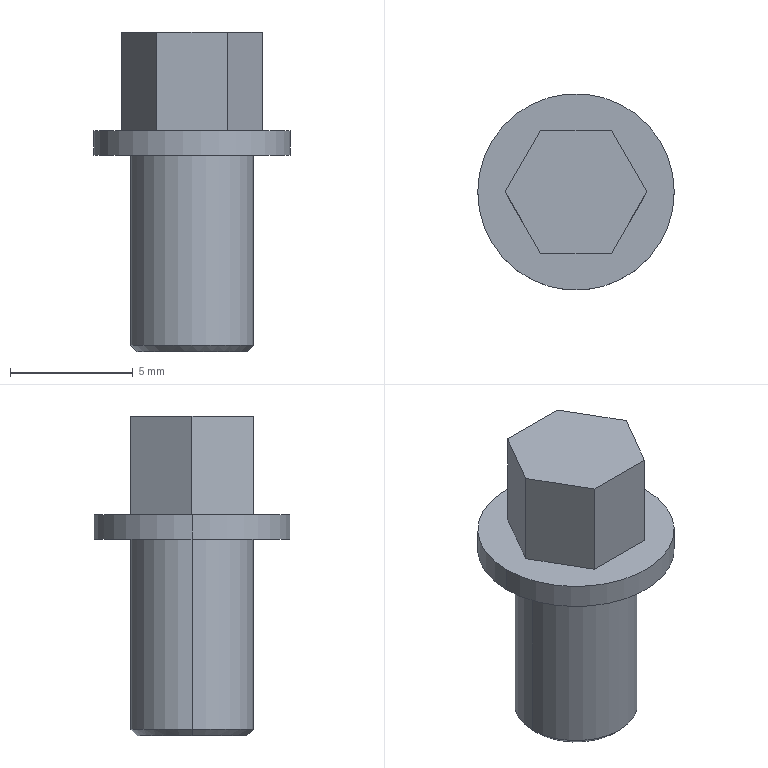Part | SolidWorks | features BaseBody 1 | 1 solid | 16 faces | box 8 x 8 x 13 mm | volume 293.473 mm3 | plane 10 | cylinder 4 | cone 2 | commonest cylinder face diameters 5 x2 8 x2
STEP:
#1=CARTESIAN_POINT('',(2.25,0.,-8.));
#2=VERTEX_POINT('',#1);
#3=CARTESIAN_POINT('',(-2.25,0.,-8.));
#4=VERTEX_POINT('',#3);
#5=CARTESIAN_POINT('',(0.,0.,-8.));
#6=DIRECTION('',(0.,0.,1.));
#7=DIRECTION('',(1.,0.,0.));
#8=AXIS2_PLACEMENT_3D('',#5,#6,#7);
#9=CIRCLE('',#8,2.25);
#10=EDGE_CURVE('',#2,#4,#9,.T.);
#11=ORIENTED_EDGE('',*,*,#10,.T.);
#12=CARTESIAN_POINT('',(-2.5,0.,-7.75));
#13=VERTEX_POINT('',#12);
#14=CARTESIAN_POINT('',(-2.375,0.,-7.875));
#15=DIRECTION('',(-0.7071,0.,0.7071));
#16=VECTOR('',#15,1000.);
#17=LINE('',#14,#16);
#18=EDGE_CURVE('',#4,#13,#17,.T.);
#19=ORIENTED_EDGE('',*,*,#18,.T.);
#20=CARTESIAN_POINT('',(2.5,0.,-7.75));
#21=VERTEX_POINT('',#20);
#22=CARTESIAN_POINT('',(0.,0.,-7.75));
#23=DIRECTION('',(0.,0.,-1.));
#24=DIRECTION('',(1.,0.,0.));
#25=AXIS2_PLACEMENT_3D('',#22,#23,#24);
#26=CIRCLE('',#25,2.5);
#27=EDGE_CURVE('',#13,#21,#26,.T.);
#28=ORIENTED_EDGE('',*,*,#27,.T.);
#29=CARTESIAN_POINT('',(2.375,0.,-7.875));
#30=DIRECTION('',(0.7071,0.,0.7071));
#31=VECTOR('',#30,1000.);
#32=LINE('',#29,#31);
#33=EDGE_CURVE('',#2,#21,#32,.T.);
#34=ORIENTED_EDGE('',*,*,#33,.F.);
#35=EDGE_LOOP('',(#11,#19,#28,#34));
#36=FACE_OUTER_BOUND('',#35,.T.);
#37=CARTESIAN_POINT('',(0.,0.,-7.875));
#38=DIRECTION('',(0.,0.,1.));
#39=DIRECTION('',(1.,0.,0.));
#40=AXIS2_PLACEMENT_3D('',#37,#38,#39);
#41=CONICAL_SURFACE('',#40,2.375,0.7854);
#42=ADVANCED_FACE('',(#36),#41,.T.);
#43=ORIENTED_EDGE('',*,*,#27,.F.);
#44=CARTESIAN_POINT('',(-2.5,0.,0.));
#45=VERTEX_POINT('',#44);
#46=CARTESIAN_POINT('',(-2.5,0.,0.));
#47=DIRECTION('',(0.,0.,1.));
#48=VECTOR('',#47,1000.);
#49=LINE('',#46,#48);
#50=EDGE_CURVE('',#13,#45,#49,.T.);
#51=ORIENTED_EDGE('',*,*,#50,.T.);
#52=CARTESIAN_POINT('',(2.5,0.,0.));
#53=VERTEX_POINT('',#52);
#54=CARTESIAN_POINT('',(0.,0.,0.));
#55=DIRECTION('',(0.,0.,1.));
#56=DIRECTION('',(1.,0.,0.));
#57=AXIS2_PLACEMENT_3D('',#54,#55,#56);
#58=CIRCLE('',#57,2.5);
#59=EDGE_CURVE('',#53,#45,#58,.T.);
#60=ORIENTED_EDGE('',*,*,#59,.F.);
#61=CARTESIAN_POINT('',(2.5,0.,0.));
#62=DIRECTION('',(0.,0.,1.));
#63=VECTOR('',#62,1000.);
#64=LINE('',#61,#63);
#65=EDGE_CURVE('',#21,#53,#64,.T.);
#66=ORIENTED_EDGE('',*,*,#65,.F.);
#67=EDGE_LOOP('',(#43,#51,#60,#66));
#68=FACE_OUTER_BOUND('',#67,.T.);
#69=CARTESIAN_POINT('',(0.,0.,0.));
#70=DIRECTION('',(0.,0.,1.));
#71=DIRECTION('',(1.,0.,0.));
#72=AXIS2_PLACEMENT_3D('',#69,#70,#71);
#73=CYLINDRICAL_SURFACE('',#72,2.5);
#74=ADVANCED_FACE('',(#68),#73,.T.);
#75=CARTESIAN_POINT('',(4.,0.,1.));
#76=VERTEX_POINT('',#75);
#77=CARTESIAN_POINT('',(-4.,0.,1.));
#78=VERTEX_POINT('',#77);
#79=CARTESIAN_POINT('',(0.,0.,1.));
#80=DIRECTION('',(0.,0.,1.));
#81=DIRECTION('',(-1.,0.,0.));
#82=AXIS2_PLACEMENT_3D('',#79,#80,#81);
#83=CIRCLE('',#82,4.);
#84=EDGE_CURVE('',#76,#78,#83,.T.);
#85=ORIENTED_EDGE('',*,*,#84,.F.);
#86=CARTESIAN_POINT('',(4.,0.,0.));
#87=VERTEX_POINT('',#86);
#88=CARTESIAN_POINT('',(4.,0.,0.));
#89=DIRECTION('',(0.,0.,-1.));
#90=VECTOR('',#89,1000.);
#91=LINE('',#88,#90);
#92=EDGE_CURVE('',#76,#87,#91,.T.);
#93=ORIENTED_EDGE('',*,*,#92,.T.);
#94=CARTESIAN_POINT('',(-4.,0.,0.));
#95=VERTEX_POINT('',#94);
#96=CARTESIAN_POINT('',(0.,0.,0.));
#97=DIRECTION('',(0.,0.,-1.));
#98=DIRECTION('',(-1.,0.,0.));
#99=AXIS2_PLACEMENT_3D('',#96,#97,#98);
#100=CIRCLE('',#99,4.);
#101=EDGE_CURVE('',#95,#87,#100,.T.);
#102=ORIENTED_EDGE('',*,*,#101,.F.);
#103=CARTESIAN_POINT('',(-4.,0.,0.));
#104=DIRECTION('',(0.,0.,-1.));
#105=VECTOR('',#104,1000.);
#106=LINE('',#103,#105);
#107=EDGE_CURVE('',#78,#95,#106,.T.);
#108=ORIENTED_EDGE('',*,*,#107,.F.);
#109=EDGE_LOOP('',(#85,#93,#102,#108));
#110=FACE_OUTER_BOUND('',#109,.T.);
#111=CARTESIAN_POINT('',(0.,0.,0.));
#112=DIRECTION('',(0.,0.,-1.));
#113=DIRECTION('',(-1.,0.,0.));
#114=AXIS2_PLACEMENT_3D('',#111,#112,#113);
#115=CYLINDRICAL_SURFACE('',#114,4.);
#116=ADVANCED_FACE('',(#110),#115,.T.);
#117=ORIENTED_EDGE('',*,*,#10,.F.);
#118=CARTESIAN_POINT('',(0.,0.,-8.));
#119=DIRECTION('',(0.,0.,1.));
#120=DIRECTION('',(1.,0.,0.));
#121=AXIS2_PLACEMENT_3D('',#118,#119,#120);
#122=CIRCLE('',#121,2.25);
#123=EDGE_CURVE('',#4,#2,#122,.T.);
#124=ORIENTED_EDGE('',*,*,#123,.F.);
#125=EDGE_LOOP('',(#117,#124));
#126=FACE_OUTER_BOUND('',#125,.T.);
#127=CARTESIAN_POINT('',(0.,0.,-8.));
#128=DIRECTION('',(0.,0.,1.));
#129=DIRECTION('',(1.,0.,0.));
#130=AXIS2_PLACEMENT_3D('',#127,#128,#129);
#131=PLANE('',#130);
#132=ADVANCED_FACE('',(#126),#131,.F.);
#133=CARTESIAN_POINT('',(-1.443,-2.5,1.));
#134=VERTEX_POINT('',#133);
#135=CARTESIAN_POINT('',(-2.887,0.,1.));
#136=VERTEX_POINT('',#135);
#137=CARTESIAN_POINT('',(-2.526,-0.625,1.));
#138=DIRECTION('',(-0.5,0.866,0.));
#139=VECTOR('',#138,1000.);
#140=LINE('',#137,#139);
#141=EDGE_CURVE('',#134,#136,#140,.T.);
#142=ORIENTED_EDGE('',*,*,#141,.F.);
#143=CARTESIAN_POINT('',(-1.443,-2.5,5.));
#144=VERTEX_POINT('',#143);
#145=CARTESIAN_POINT('',(-1.443,-2.5,1.));
#146=DIRECTION('',(0.,0.,1.));
#147=VECTOR('',#146,1000.);
#148=LINE('',#145,#147);
#149=EDGE_CURVE('',#134,#144,#148,.T.);
#150=ORIENTED_EDGE('',*,*,#149,.T.);
#151=CARTESIAN_POINT('',(-2.887,0.,5.));
#152=VERTEX_POINT('',#151);
#153=CARTESIAN_POINT('',(-1.443,-2.5,5.));
#154=DIRECTION('',(0.5,-0.866,0.));
#155=VECTOR('',#154,1000.);
#156=LINE('',#153,#155);
#157=EDGE_CURVE('',#152,#144,#156,.T.);
#158=ORIENTED_EDGE('',*,*,#157,.F.);
#159=CARTESIAN_POINT('',(-2.887,0.,1.));
#160=DIRECTION('',(0.,0.,1.));
#161=VECTOR('',#160,1000.);
#162=LINE('',#159,#161);
#163=EDGE_CURVE('',#136,#152,#162,.T.);
#164=ORIENTED_EDGE('',*,*,#163,.F.);
#165=EDGE_LOOP('',(#142,#150,#158,#164));
#166=FACE_OUTER_BOUND('',#165,.T.);
#167=CARTESIAN_POINT('',(-2.887,0.,1.));
#168=DIRECTION('',(-0.866,-0.5,0.));
#169=DIRECTION('',(-0.5,0.866,0.));
#170=AXIS2_PLACEMENT_3D('',#167,#168,#169);
#171=PLANE('',#170);
#172=ADVANCED_FACE('',(#166),#171,.T.);
#173=CARTESIAN_POINT('',(-1.443,2.5,1.));
#174=VERTEX_POINT('',#173);
#175=CARTESIAN_POINT('',(-1.804,1.875,1.));
#176=DIRECTION('',(0.5,0.866,0.));
#177=VECTOR('',#176,1000.);
#178=LINE('',#175,#177);
#179=EDGE_CURVE('',#136,#174,#178,.T.);
#180=ORIENTED_EDGE('',*,*,#179,.F.);
#181=ORIENTED_EDGE('',*,*,#163,.T.);
#182=CARTESIAN_POINT('',(-1.443,2.5,5.));
#183=VERTEX_POINT('',#182);
#184=CARTESIAN_POINT('',(-2.887,0.,5.));
#185=DIRECTION('',(-0.5,-0.866,0.));
#186=VECTOR('',#185,1000.);
#187=LINE('',#184,#186);
#188=EDGE_CURVE('',#183,#152,#187,.T.);
#189=ORIENTED_EDGE('',*,*,#188,.F.);
#190=CARTESIAN_POINT('',(-1.443,2.5,1.));
#191=DIRECTION('',(0.,0.,1.));
#192=VECTOR('',#191,1000.);
#193=LINE('',#190,#192);
#194=EDGE_CURVE('',#174,#183,#193,.T.);
#195=ORIENTED_EDGE('',*,*,#194,.F.);
#196=EDGE_LOOP('',(#180,#181,#189,#195));
#197=FACE_OUTER_BOUND('',#196,.T.);
#198=CARTESIAN_POINT('',(-1.443,2.5,1.));
#199=DIRECTION('',(-0.866,0.5,0.));
#200=DIRECTION('',(0.,0.,1.));
#201=AXIS2_PLACEMENT_3D('',#198,#199,#200);
#202=PLANE('',#201);
#203=ADVANCED_FACE('',(#197),#202,.T.);
#204=CARTESIAN_POINT('',(1.443,2.5,1.));
#205=VERTEX_POINT('',#204);
#206=CARTESIAN_POINT('',(0.7217,2.5,1.));
#207=DIRECTION('',(1.,0.,0.));
#208=VECTOR('',#207,1000.);
#209=LINE('',#206,#208);
#210=EDGE_CURVE('',#174,#205,#209,.T.);
#211=ORIENTED_EDGE('',*,*,#210,.F.);
#212=ORIENTED_EDGE('',*,*,#194,.T.);
#213=CARTESIAN_POINT('',(1.443,2.5,5.));
#214=VERTEX_POINT('',#213);
#215=CARTESIAN_POINT('',(-1.443,2.5,5.));
#216=DIRECTION('',(-1.,0.,0.));
#217=VECTOR('',#216,1000.);
#218=LINE('',#215,#217);
#219=EDGE_CURVE('',#214,#183,#218,.T.);
#220=ORIENTED_EDGE('',*,*,#219,.F.);
#221=CARTESIAN_POINT('',(1.443,2.5,1.));
#222=DIRECTION('',(0.,0.,1.));
#223=VECTOR('',#222,1000.);
#224=LINE('',#221,#223);
#225=EDGE_CURVE('',#205,#214,#224,.T.);
#226=ORIENTED_EDGE('',*,*,#225,.F.);
#227=EDGE_LOOP('',(#211,#212,#220,#226));
#228=FACE_OUTER_BOUND('',#227,.T.);
#229=CARTESIAN_POINT('',(1.443,2.5,1.));
#230=DIRECTION('',(0.,1.,0.));
#231=DIRECTION('',(1.,0.,0.));
#232=AXIS2_PLACEMENT_3D('',#229,#230,#231);
#233=PLANE('',#232);
#234=ADVANCED_FACE('',(#228),#233,.T.);
#235=CARTESIAN_POINT('',(2.887,0.,1.));
#236=VERTEX_POINT('',#235);
#237=CARTESIAN_POINT('',(2.526,0.625,1.));
#238=DIRECTION('',(0.5,-0.866,0.));
#239=VECTOR('',#238,1000.);
#240=LINE('',#237,#239);
#241=EDGE_CURVE('',#205,#236,#240,.T.);
#242=ORIENTED_EDGE('',*,*,#241,.F.);
#243=ORIENTED_EDGE('',*,*,#225,.T.);
#244=CARTESIAN_POINT('',(2.887,0.,5.));
#245=VERTEX_POINT('',#244);
#246=CARTESIAN_POINT('',(1.443,2.5,5.));
#247=DIRECTION('',(-0.5,0.866,0.));
#248=VECTOR('',#247,1000.);
#249=LINE('',#246,#248);
#250=EDGE_CURVE('',#245,#214,#249,.T.);
#251=ORIENTED_EDGE('',*,*,#250,.F.);
#252=CARTESIAN_POINT('',(2.887,0.,1.));
#253=DIRECTION('',(0.,0.,1.));
#254=VECTOR('',#253,1000.);
#255=LINE('',#252,#254);
#256=EDGE_CURVE('',#236,#245,#255,.T.);
#257=ORIENTED_EDGE('',*,*,#256,.F.);
#258=EDGE_LOOP('',(#242,#243,#251,#257));
#259=FACE_OUTER_BOUND('',#258,.T.);
#260=CARTESIAN_POINT('',(2.887,0.,1.));
#261=DIRECTION('',(0.866,0.5,0.));
#262=DIRECTION('',(0.,0.,-1.));
#263=AXIS2_PLACEMENT_3D('',#260,#261,#262);
#264=PLANE('',#263);
#265=ADVANCED_FACE('',(#259),#264,.T.);
#266=CARTESIAN_POINT('',(1.443,-2.5,1.));
#267=VERTEX_POINT('',#266);
#268=CARTESIAN_POINT('',(1.804,-1.875,1.));
#269=DIRECTION('',(-0.5,-0.866,0.));
#270=VECTOR('',#269,1000.);
#271=LINE('',#268,#270);
#272=EDGE_CURVE('',#236,#267,#271,.T.);
#273=ORIENTED_EDGE('',*,*,#272,.F.);
#274=ORIENTED_EDGE('',*,*,#256,.T.);
#275=CARTESIAN_POINT('',(1.443,-2.5,5.));
#276=VERTEX_POINT('',#275);
#277=CARTESIAN_POINT('',(2.887,0.,5.));
#278=DIRECTION('',(0.5,0.866,0.));
#279=VECTOR('',#278,1000.);
#280=LINE('',#277,#279);
#281=EDGE_CURVE('',#276,#245,#280,.T.);
#282=ORIENTED_EDGE('',*,*,#281,.F.);
#283=CARTESIAN_POINT('',(1.443,-2.5,1.));
#284=DIRECTION('',(0.,0.,1.));
#285=VECTOR('',#284,1000.);
#286=LINE('',#283,#285);
#287=EDGE_CURVE('',#267,#276,#286,.T.);
#288=ORIENTED_EDGE('',*,*,#287,.F.);
#289=EDGE_LOOP('',(#273,#274,#282,#288));
#290=FACE_OUTER_BOUND('',#289,.T.);
#291=CARTESIAN_POINT('',(1.443,-2.5,1.));
#292=DIRECTION('',(0.866,-0.5,0.));
#293=DIRECTION('',(0.,0.,-1.));
#294=AXIS2_PLACEMENT_3D('',#291,#292,#293);
#295=PLANE('',#294);
#296=ADVANCED_FACE('',(#290),#295,.T.);
#297=CARTESIAN_POINT('',(-0.7217,-2.5,1.));
#298=DIRECTION('',(-1.,0.,0.));
#299=VECTOR('',#298,1000.);
#300=LINE('',#297,#299);
#301=EDGE_CURVE('',#267,#134,#300,.T.);
#302=ORIENTED_EDGE('',*,*,#301,.F.);
#303=ORIENTED_EDGE('',*,*,#287,.T.);
#304=CARTESIAN_POINT('',(1.443,-2.5,5.));
#305=DIRECTION('',(1.,0.,0.));
#306=VECTOR('',#305,1000.);
#307=LINE('',#304,#306);
#308=EDGE_CURVE('',#144,#276,#307,.T.);
#309=ORIENTED_EDGE('',*,*,#308,.F.);
#310=ORIENTED_EDGE('',*,*,#149,.F.);
#311=EDGE_LOOP('',(#302,#303,#309,#310));
#312=FACE_OUTER_BOUND('',#311,.T.);
#313=CARTESIAN_POINT('',(-1.443,-2.5,1.));
#314=DIRECTION('',(0.,-1.,0.));
#315=DIRECTION('',(-1.,0.,0.));
#316=AXIS2_PLACEMENT_3D('',#313,#314,#315);
#317=PLANE('',#316);
#318=ADVANCED_FACE('',(#312),#317,.T.);
#319=ORIENTED_EDGE('',*,*,#308,.T.);
#320=ORIENTED_EDGE('',*,*,#281,.T.);
#321=ORIENTED_EDGE('',*,*,#250,.T.);
#322=ORIENTED_EDGE('',*,*,#219,.T.);
#323=ORIENTED_EDGE('',*,*,#188,.T.);
#324=ORIENTED_EDGE('',*,*,#157,.T.);
#325=EDGE_LOOP('',(#319,#320,#321,#322,#323,#324));
#326=FACE_OUTER_BOUND('',#325,.T.);
#327=CARTESIAN_POINT('',(0.,0.,5.));
#328=DIRECTION('',(0.,0.,1.));
#329=DIRECTION('',(1.,0.,0.));
#330=AXIS2_PLACEMENT_3D('',#327,#328,#329);
#331=PLANE('',#330);
#332=ADVANCED_FACE('',(#326),#331,.T.);
#333=ORIENTED_EDGE('',*,*,#59,.T.);
#334=CARTESIAN_POINT('',(0.,0.,0.));
#335=DIRECTION('',(0.,0.,1.));
#336=DIRECTION('',(1.,0.,0.));
#337=AXIS2_PLACEMENT_3D('',#334,#335,#336);
#338=CIRCLE('',#337,2.5);
#339=EDGE_CURVE('',#45,#53,#338,.T.);
#340=ORIENTED_EDGE('',*,*,#339,.T.);
#341=EDGE_LOOP('',(#333,#340));
#342=FACE_BOUND('',#341,.T.);
#343=ORIENTED_EDGE('',*,*,#101,.T.);
#344=CARTESIAN_POINT('',(0.,0.,0.));
#345=DIRECTION('',(0.,0.,-1.));
#346=DIRECTION('',(-1.,0.,0.));
#347=AXIS2_PLACEMENT_3D('',#344,#345,#346);
#348=CIRCLE('',#347,4.);
#349=EDGE_CURVE('',#87,#95,#348,.T.);
#350=ORIENTED_EDGE('',*,*,#349,.T.);
#351=EDGE_LOOP('',(#343,#350));
#352=FACE_OUTER_BOUND('',#351,.T.);
#353=CARTESIAN_POINT('',(0.,0.,0.));
#354=DIRECTION('',(0.,0.,1.));
#355=DIRECTION('',(1.,0.,0.));
#356=AXIS2_PLACEMENT_3D('',#353,#354,#355);
#357=PLANE('',#356);
#358=ADVANCED_FACE('',(#342,#352),#357,.F.);
#359=ORIENTED_EDGE('',*,*,#141,.T.);
#360=ORIENTED_EDGE('',*,*,#179,.T.);
#361=ORIENTED_EDGE('',*,*,#210,.T.);
#362=ORIENTED_EDGE('',*,*,#241,.T.);
#363=ORIENTED_EDGE('',*,*,#272,.T.);
#364=ORIENTED_EDGE('',*,*,#301,.T.);
#365=EDGE_LOOP('',(#359,#360,#361,#362,#363,#364));
#366=FACE_BOUND('',#365,.T.);
#367=CARTESIAN_POINT('',(0.,0.,1.));
#368=DIRECTION('',(0.,0.,1.));
#369=DIRECTION('',(-1.,0.,0.));
#370=AXIS2_PLACEMENT_3D('',#367,#368,#369);
#371=CIRCLE('',#370,4.);
#372=EDGE_CURVE('',#78,#76,#371,.T.);
#373=ORIENTED_EDGE('',*,*,#372,.T.);
#374=ORIENTED_EDGE('',*,*,#84,.T.);
#375=EDGE_LOOP('',(#373,#374));
#376=FACE_OUTER_BOUND('',#375,.T.);
#377=CARTESIAN_POINT('',(0.,0.,1.));
#378=DIRECTION('',(0.,0.,1.));
#379=DIRECTION('',(1.,0.,0.));
#380=AXIS2_PLACEMENT_3D('',#377,#378,#379);
#381=PLANE('',#380);
#382=ADVANCED_FACE('',(#366,#376),#381,.T.);
#383=ORIENTED_EDGE('',*,*,#92,.F.);
#384=ORIENTED_EDGE('',*,*,#372,.F.);
#385=ORIENTED_EDGE('',*,*,#107,.T.);
#386=ORIENTED_EDGE('',*,*,#349,.F.);
#387=EDGE_LOOP('',(#383,#384,#385,#386));
#388=FACE_OUTER_BOUND('',#387,.T.);
#389=CARTESIAN_POINT('',(0.,0.,0.));
#390=DIRECTION('',(0.,0.,-1.));
#391=DIRECTION('',(-1.,0.,0.));
#392=AXIS2_PLACEMENT_3D('',#389,#390,#391);
#393=CYLINDRICAL_SURFACE('',#392,4.);
#394=ADVANCED_FACE('',(#388),#393,.T.);
#395=ORIENTED_EDGE('',*,*,#50,.F.);
#396=CARTESIAN_POINT('',(0.,0.,-7.75));
#397=DIRECTION('',(0.,0.,-1.));
#398=DIRECTION('',(1.,0.,0.));
#399=AXIS2_PLACEMENT_3D('',#396,#397,#398);
#400=CIRCLE('',#399,2.5);
#401=EDGE_CURVE('',#21,#13,#400,.T.);
#402=ORIENTED_EDGE('',*,*,#401,.F.);
#403=ORIENTED_EDGE('',*,*,#65,.T.);
#404=ORIENTED_EDGE('',*,*,#339,.F.);
#405=EDGE_LOOP('',(#395,#402,#403,#404));
#406=FACE_OUTER_BOUND('',#405,.T.);
#407=CARTESIAN_POINT('',(0.,0.,0.));
#408=DIRECTION('',(0.,0.,1.));
#409=DIRECTION('',(1.,0.,0.));
#410=AXIS2_PLACEMENT_3D('',#407,#408,#409);
#411=CYLINDRICAL_SURFACE('',#410,2.5);
#412=ADVANCED_FACE('',(#406),#411,.T.);
#413=ORIENTED_EDGE('',*,*,#18,.F.);
#414=ORIENTED_EDGE('',*,*,#123,.T.);
#415=ORIENTED_EDGE('',*,*,#33,.T.);
#416=ORIENTED_EDGE('',*,*,#401,.T.);
#417=EDGE_LOOP('',(#413,#414,#415,#416));
#418=FACE_OUTER_BOUND('',#417,.T.);
#419=CARTESIAN_POINT('',(0.,0.,-7.875));
#420=DIRECTION('',(0.,0.,1.));
#421=DIRECTION('',(1.,0.,0.));
#422=AXIS2_PLACEMENT_3D('',#419,#420,#421);
#423=CONICAL_SURFACE('',#422,2.375,0.7854);
#424=ADVANCED_FACE('',(#418),#423,.T.);
#425=CLOSED_SHELL('',(#42,#74,#116,#132,#172,#203,#234,#265,#296,#318,#332,#358,#382,#394,#412,#424));
#426=MANIFOLD_SOLID_BREP('',#425);
#427=CARTESIAN_POINT('',(0.,0.,0.));
#428=DIRECTION('',(0.,0.,1.));
#429=DIRECTION('',(1.,0.,0.));
#430=AXIS2_PLACEMENT_3D('',#427,#428,#429);
#431=(LENGTH_UNIT()NAMED_UNIT(*)SI_UNIT(.MILLI.,.METRE.));
#432=UNCERTAINTY_MEASURE_WITH_UNIT(LENGTH_MEASURE(0.00001),#431,'','');
#433=(NAMED_UNIT(*)PLANE_ANGLE_UNIT()SI_UNIT($,.RADIAN.));
#434=(NAMED_UNIT(*)SI_UNIT($,.STERADIAN.)SOLID_ANGLE_UNIT());
#435=(GEOMETRIC_REPRESENTATION_CONTEXT(3)GLOBAL_UNCERTAINTY_ASSIGNED_CONTEXT((#432))GLOBAL_UNIT_ASSIGNED_CONTEXT((#431,#433,#434))REPRESENTATION_CONTEXT('',''));
#436=ADVANCED_BREP_SHAPE_REPRESENTATION('',(#426,#430),#435);